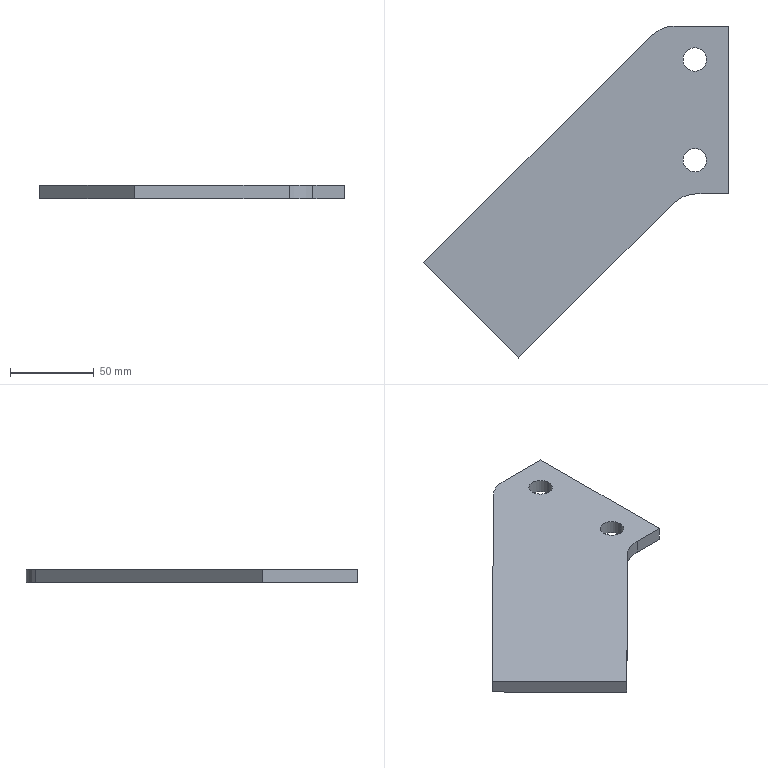Part | SolidWorks | features Extrusion 1 | 1 solid | 14 faces | box 181.644 x 197.856 x 8 mm | volume 132691 mm3 | plane 8 | cylinder 6 | commonest cylinder face diameters 14 x4 40 x2
STEP:
#1=CARTESIAN_POINT('',(-27.,-80.,8.));
#2=VERTEX_POINT('',#1);
#3=CARTESIAN_POINT('',(-13.,-80.,8.));
#4=VERTEX_POINT('',#3);
#5=CARTESIAN_POINT('',(-20.,-80.,8.));
#6=DIRECTION('',(0.,0.,1.));
#7=DIRECTION('',(1.,0.,0.));
#8=AXIS2_PLACEMENT_3D('',#5,#6,#7);
#9=CIRCLE('',#8,7.);
#10=EDGE_CURVE('',#2,#4,#9,.T.);
#11=ORIENTED_EDGE('',*,*,#10,.T.);
#12=CARTESIAN_POINT('',(-13.,-80.,0.));
#13=VERTEX_POINT('',#12);
#14=CARTESIAN_POINT('',(-13.,-80.,8.));
#15=DIRECTION('',(0.,0.,-1.));
#16=VECTOR('',#15,1000.);
#17=LINE('',#14,#16);
#18=EDGE_CURVE('',#4,#13,#17,.T.);
#19=ORIENTED_EDGE('',*,*,#18,.T.);
#20=CARTESIAN_POINT('',(-27.,-80.,0.));
#21=VERTEX_POINT('',#20);
#22=CARTESIAN_POINT('',(-20.,-80.,0.));
#23=DIRECTION('',(0.,0.,1.));
#24=DIRECTION('',(1.,0.,0.));
#25=AXIS2_PLACEMENT_3D('',#22,#23,#24);
#26=CIRCLE('',#25,7.);
#27=EDGE_CURVE('',#21,#13,#26,.T.);
#28=ORIENTED_EDGE('',*,*,#27,.F.);
#29=CARTESIAN_POINT('',(-27.,-80.,8.));
#30=DIRECTION('',(0.,0.,-1.));
#31=VECTOR('',#30,1000.);
#32=LINE('',#29,#31);
#33=EDGE_CURVE('',#2,#21,#32,.T.);
#34=ORIENTED_EDGE('',*,*,#33,.F.);
#35=EDGE_LOOP('',(#11,#19,#28,#34));
#36=FACE_OUTER_BOUND('',#35,.T.);
#37=CARTESIAN_POINT('',(-20.,-80.,8.));
#38=DIRECTION('',(0.,0.,-1.));
#39=DIRECTION('',(-1.,0.,0.));
#40=AXIS2_PLACEMENT_3D('',#37,#38,#39);
#41=CYLINDRICAL_SURFACE('',#40,7.);
#42=ADVANCED_FACE('',(#36),#41,.F.);
#43=CARTESIAN_POINT('',(-27.,-20.,8.));
#44=VERTEX_POINT('',#43);
#45=CARTESIAN_POINT('',(-13.,-20.,8.));
#46=VERTEX_POINT('',#45);
#47=CARTESIAN_POINT('',(-20.,-20.,8.));
#48=DIRECTION('',(0.,0.,1.));
#49=DIRECTION('',(1.,0.,0.));
#50=AXIS2_PLACEMENT_3D('',#47,#48,#49);
#51=CIRCLE('',#50,7.);
#52=EDGE_CURVE('',#44,#46,#51,.T.);
#53=ORIENTED_EDGE('',*,*,#52,.T.);
#54=CARTESIAN_POINT('',(-13.,-20.,0.));
#55=VERTEX_POINT('',#54);
#56=CARTESIAN_POINT('',(-13.,-20.,8.));
#57=DIRECTION('',(0.,0.,-1.));
#58=VECTOR('',#57,1000.);
#59=LINE('',#56,#58);
#60=EDGE_CURVE('',#46,#55,#59,.T.);
#61=ORIENTED_EDGE('',*,*,#60,.T.);
#62=CARTESIAN_POINT('',(-27.,-20.,0.));
#63=VERTEX_POINT('',#62);
#64=CARTESIAN_POINT('',(-20.,-20.,0.));
#65=DIRECTION('',(0.,0.,1.));
#66=DIRECTION('',(1.,0.,0.));
#67=AXIS2_PLACEMENT_3D('',#64,#65,#66);
#68=CIRCLE('',#67,7.);
#69=EDGE_CURVE('',#63,#55,#68,.T.);
#70=ORIENTED_EDGE('',*,*,#69,.F.);
#71=CARTESIAN_POINT('',(-27.,-20.,8.));
#72=DIRECTION('',(0.,0.,-1.));
#73=VECTOR('',#72,1000.);
#74=LINE('',#71,#73);
#75=EDGE_CURVE('',#44,#63,#74,.T.);
#76=ORIENTED_EDGE('',*,*,#75,.F.);
#77=EDGE_LOOP('',(#53,#61,#70,#76));
#78=FACE_OUTER_BOUND('',#77,.T.);
#79=CARTESIAN_POINT('',(-20.,-20.,8.));
#80=DIRECTION('',(0.,0.,-1.));
#81=DIRECTION('',(-1.,0.,0.));
#82=AXIS2_PLACEMENT_3D('',#79,#80,#81);
#83=CYLINDRICAL_SURFACE('',#82,7.);
#84=ADVANCED_FACE('',(#78),#83,.F.);
#85=CARTESIAN_POINT('',(0.,-100.,8.));
#86=VERTEX_POINT('',#85);
#87=CARTESIAN_POINT('',(0.,0.,8.));
#88=VERTEX_POINT('',#87);
#89=CARTESIAN_POINT('',(0.,0.,8.));
#90=DIRECTION('',(0.,1.,0.));
#91=VECTOR('',#90,1000.);
#92=LINE('',#89,#91);
#93=EDGE_CURVE('',#86,#88,#92,.T.);
#94=ORIENTED_EDGE('',*,*,#93,.T.);
#95=CARTESIAN_POINT('',(-31.734,0.,8.));
#96=VERTEX_POINT('',#95);
#97=CARTESIAN_POINT('',(0.,0.,8.));
#98=DIRECTION('',(-1.,0.,0.));
#99=VECTOR('',#98,1000.);
#100=LINE('',#97,#99);
#101=EDGE_CURVE('',#88,#96,#100,.T.);
#102=ORIENTED_EDGE('',*,*,#101,.T.);
#103=CARTESIAN_POINT('',(-45.854,-5.836,8.));
#104=VERTEX_POINT('',#103);
#105=CARTESIAN_POINT('',(-31.734,-20.,8.));
#106=DIRECTION('',(0.,0.,1.));
#107=DIRECTION('',(1.,0.,0.));
#108=AXIS2_PLACEMENT_3D('',#105,#106,#107);
#109=CIRCLE('',#108,20.);
#110=EDGE_CURVE('',#96,#104,#109,.T.);
#111=ORIENTED_EDGE('',*,*,#110,.T.);
#112=CARTESIAN_POINT('',(-181.644,-141.198,8.));
#113=VERTEX_POINT('',#112);
#114=CARTESIAN_POINT('',(-45.854,-5.836,8.));
#115=DIRECTION('',(-0.7082,-0.706,0.));
#116=VECTOR('',#115,1000.);
#117=LINE('',#114,#116);
#118=EDGE_CURVE('',#104,#113,#117,.T.);
#119=ORIENTED_EDGE('',*,*,#118,.T.);
#120=CARTESIAN_POINT('',(-125.165,-197.856,8.));
#121=VERTEX_POINT('',#120);
#122=CARTESIAN_POINT('',(-181.644,-141.198,8.));
#123=DIRECTION('',(0.706,-0.7082,0.));
#124=VECTOR('',#123,1000.);
#125=LINE('',#122,#124);
#126=EDGE_CURVE('',#113,#121,#125,.T.);
#127=ORIENTED_EDGE('',*,*,#126,.T.);
#128=CARTESIAN_POINT('',(-32.854,-105.836,8.));
#129=VERTEX_POINT('',#128);
#130=CARTESIAN_POINT('',(-125.165,-197.856,8.));
#131=DIRECTION('',(0.7082,0.706,0.));
#132=VECTOR('',#131,1000.);
#133=LINE('',#130,#132);
#134=EDGE_CURVE('',#121,#129,#133,.T.);
#135=ORIENTED_EDGE('',*,*,#134,.T.);
#136=CARTESIAN_POINT('',(-18.734,-100.,8.));
#137=VERTEX_POINT('',#136);
#138=CARTESIAN_POINT('',(-18.734,-120.,8.));
#139=DIRECTION('',(0.,0.,-1.));
#140=DIRECTION('',(-1.,0.,0.));
#141=AXIS2_PLACEMENT_3D('',#138,#139,#140);
#142=CIRCLE('',#141,20.);
#143=EDGE_CURVE('',#129,#137,#142,.T.);
#144=ORIENTED_EDGE('',*,*,#143,.T.);
#145=CARTESIAN_POINT('',(0.,-100.,8.));
#146=DIRECTION('',(1.,0.,0.));
#147=VECTOR('',#146,1000.);
#148=LINE('',#145,#147);
#149=EDGE_CURVE('',#137,#86,#148,.T.);
#150=ORIENTED_EDGE('',*,*,#149,.T.);
#151=EDGE_LOOP('',(#94,#102,#111,#119,#127,#135,#144,#150));
#152=FACE_OUTER_BOUND('',#151,.T.);
#153=ORIENTED_EDGE('',*,*,#52,.F.);
#154=CARTESIAN_POINT('',(-20.,-20.,8.));
#155=DIRECTION('',(0.,0.,1.));
#156=DIRECTION('',(1.,0.,0.));
#157=AXIS2_PLACEMENT_3D('',#154,#155,#156);
#158=CIRCLE('',#157,7.);
#159=EDGE_CURVE('',#46,#44,#158,.T.);
#160=ORIENTED_EDGE('',*,*,#159,.F.);
#161=EDGE_LOOP('',(#153,#160));
#162=FACE_BOUND('',#161,.T.);
#163=ORIENTED_EDGE('',*,*,#10,.F.);
#164=CARTESIAN_POINT('',(-20.,-80.,8.));
#165=DIRECTION('',(0.,0.,1.));
#166=DIRECTION('',(1.,0.,0.));
#167=AXIS2_PLACEMENT_3D('',#164,#165,#166);
#168=CIRCLE('',#167,7.);
#169=EDGE_CURVE('',#4,#2,#168,.T.);
#170=ORIENTED_EDGE('',*,*,#169,.F.);
#171=EDGE_LOOP('',(#163,#170));
#172=FACE_BOUND('',#171,.T.);
#173=CARTESIAN_POINT('',(-18.734,-120.,8.));
#174=DIRECTION('',(0.,0.,-1.));
#175=DIRECTION('',(-1.,0.,0.));
#176=AXIS2_PLACEMENT_3D('',#173,#174,#175);
#177=PLANE('',#176);
#178=ADVANCED_FACE('',(#152,#162,#172),#177,.F.);
#179=ORIENTED_EDGE('',*,*,#69,.T.);
#180=CARTESIAN_POINT('',(-20.,-20.,0.));
#181=DIRECTION('',(0.,0.,1.));
#182=DIRECTION('',(1.,0.,0.));
#183=AXIS2_PLACEMENT_3D('',#180,#181,#182);
#184=CIRCLE('',#183,7.);
#185=EDGE_CURVE('',#55,#63,#184,.T.);
#186=ORIENTED_EDGE('',*,*,#185,.T.);
#187=EDGE_LOOP('',(#179,#186));
#188=FACE_BOUND('',#187,.T.);
#189=CARTESIAN_POINT('',(0.,-100.,0.));
#190=VERTEX_POINT('',#189);
#191=CARTESIAN_POINT('',(0.,0.,0.));
#192=VERTEX_POINT('',#191);
#193=CARTESIAN_POINT('',(0.,0.,0.));
#194=DIRECTION('',(0.,1.,0.));
#195=VECTOR('',#194,1000.);
#196=LINE('',#193,#195);
#197=EDGE_CURVE('',#190,#192,#196,.T.);
#198=ORIENTED_EDGE('',*,*,#197,.F.);
#199=CARTESIAN_POINT('',(-18.734,-100.,0.));
#200=VERTEX_POINT('',#199);
#201=CARTESIAN_POINT('',(0.,-100.,0.));
#202=DIRECTION('',(1.,0.,0.));
#203=VECTOR('',#202,1000.);
#204=LINE('',#201,#203);
#205=EDGE_CURVE('',#200,#190,#204,.T.);
#206=ORIENTED_EDGE('',*,*,#205,.F.);
#207=CARTESIAN_POINT('',(-32.854,-105.836,0.));
#208=VERTEX_POINT('',#207);
#209=CARTESIAN_POINT('',(-18.734,-120.,0.));
#210=DIRECTION('',(0.,0.,-1.));
#211=DIRECTION('',(-1.,0.,0.));
#212=AXIS2_PLACEMENT_3D('',#209,#210,#211);
#213=CIRCLE('',#212,20.);
#214=EDGE_CURVE('',#208,#200,#213,.T.);
#215=ORIENTED_EDGE('',*,*,#214,.F.);
#216=CARTESIAN_POINT('',(-125.165,-197.856,0.));
#217=VERTEX_POINT('',#216);
#218=CARTESIAN_POINT('',(-125.165,-197.856,0.));
#219=DIRECTION('',(0.7082,0.706,0.));
#220=VECTOR('',#219,1000.);
#221=LINE('',#218,#220);
#222=EDGE_CURVE('',#217,#208,#221,.T.);
#223=ORIENTED_EDGE('',*,*,#222,.F.);
#224=CARTESIAN_POINT('',(-181.644,-141.198,0.));
#225=VERTEX_POINT('',#224);
#226=CARTESIAN_POINT('',(-181.644,-141.198,0.));
#227=DIRECTION('',(0.706,-0.7082,0.));
#228=VECTOR('',#227,1000.);
#229=LINE('',#226,#228);
#230=EDGE_CURVE('',#225,#217,#229,.T.);
#231=ORIENTED_EDGE('',*,*,#230,.F.);
#232=CARTESIAN_POINT('',(-45.854,-5.836,0.));
#233=VERTEX_POINT('',#232);
#234=CARTESIAN_POINT('',(-45.854,-5.836,0.));
#235=DIRECTION('',(-0.7082,-0.706,0.));
#236=VECTOR('',#235,1000.);
#237=LINE('',#234,#236);
#238=EDGE_CURVE('',#233,#225,#237,.T.);
#239=ORIENTED_EDGE('',*,*,#238,.F.);
#240=CARTESIAN_POINT('',(-31.734,0.,0.));
#241=VERTEX_POINT('',#240);
#242=CARTESIAN_POINT('',(-31.734,-20.,0.));
#243=DIRECTION('',(0.,0.,1.));
#244=DIRECTION('',(1.,0.,0.));
#245=AXIS2_PLACEMENT_3D('',#242,#243,#244);
#246=CIRCLE('',#245,20.);
#247=EDGE_CURVE('',#241,#233,#246,.T.);
#248=ORIENTED_EDGE('',*,*,#247,.F.);
#249=CARTESIAN_POINT('',(0.,0.,0.));
#250=DIRECTION('',(-1.,0.,0.));
#251=VECTOR('',#250,1000.);
#252=LINE('',#249,#251);
#253=EDGE_CURVE('',#192,#241,#252,.T.);
#254=ORIENTED_EDGE('',*,*,#253,.F.);
#255=EDGE_LOOP('',(#198,#206,#215,#223,#231,#239,#248,#254));
#256=FACE_OUTER_BOUND('',#255,.T.);
#257=ORIENTED_EDGE('',*,*,#27,.T.);
#258=CARTESIAN_POINT('',(-20.,-80.,0.));
#259=DIRECTION('',(0.,0.,1.));
#260=DIRECTION('',(1.,0.,0.));
#261=AXIS2_PLACEMENT_3D('',#258,#259,#260);
#262=CIRCLE('',#261,7.);
#263=EDGE_CURVE('',#13,#21,#262,.T.);
#264=ORIENTED_EDGE('',*,*,#263,.T.);
#265=EDGE_LOOP('',(#257,#264));
#266=FACE_BOUND('',#265,.T.);
#267=CARTESIAN_POINT('',(-18.734,-120.,0.));
#268=DIRECTION('',(0.,0.,-1.));
#269=DIRECTION('',(-1.,0.,0.));
#270=AXIS2_PLACEMENT_3D('',#267,#268,#269);
#271=PLANE('',#270);
#272=ADVANCED_FACE('',(#188,#256,#266),#271,.T.);
#273=ORIENTED_EDGE('',*,*,#197,.T.);
#274=CARTESIAN_POINT('',(0.,0.,8.));
#275=DIRECTION('',(0.,0.,-1.));
#276=VECTOR('',#275,1000.);
#277=LINE('',#274,#276);
#278=EDGE_CURVE('',#88,#192,#277,.T.);
#279=ORIENTED_EDGE('',*,*,#278,.F.);
#280=ORIENTED_EDGE('',*,*,#93,.F.);
#281=CARTESIAN_POINT('',(0.,-100.,8.));
#282=DIRECTION('',(0.,0.,-1.));
#283=VECTOR('',#282,1000.);
#284=LINE('',#281,#283);
#285=EDGE_CURVE('',#86,#190,#284,.T.);
#286=ORIENTED_EDGE('',*,*,#285,.T.);
#287=EDGE_LOOP('',(#273,#279,#280,#286));
#288=FACE_OUTER_BOUND('',#287,.T.);
#289=CARTESIAN_POINT('',(0.,0.,8.));
#290=DIRECTION('',(-1.,0.,0.));
#291=DIRECTION('',(0.,-1.,0.));
#292=AXIS2_PLACEMENT_3D('',#289,#290,#291);
#293=PLANE('',#292);
#294=ADVANCED_FACE('',(#288),#293,.F.);
#295=ORIENTED_EDGE('',*,*,#253,.T.);
#296=CARTESIAN_POINT('',(-31.734,0.,8.));
#297=DIRECTION('',(0.,0.,-1.));
#298=VECTOR('',#297,1000.);
#299=LINE('',#296,#298);
#300=EDGE_CURVE('',#96,#241,#299,.T.);
#301=ORIENTED_EDGE('',*,*,#300,.F.);
#302=ORIENTED_EDGE('',*,*,#101,.F.);
#303=ORIENTED_EDGE('',*,*,#278,.T.);
#304=EDGE_LOOP('',(#295,#301,#302,#303));
#305=FACE_OUTER_BOUND('',#304,.T.);
#306=CARTESIAN_POINT('',(0.,0.,8.));
#307=DIRECTION('',(0.,-1.,0.));
#308=DIRECTION('',(0.,0.,-1.));
#309=AXIS2_PLACEMENT_3D('',#306,#307,#308);
#310=PLANE('',#309);
#311=ADVANCED_FACE('',(#305),#310,.F.);
#312=ORIENTED_EDGE('',*,*,#247,.T.);
#313=CARTESIAN_POINT('',(-45.854,-5.836,8.));
#314=DIRECTION('',(0.,0.,-1.));
#315=VECTOR('',#314,1000.);
#316=LINE('',#313,#315);
#317=EDGE_CURVE('',#104,#233,#316,.T.);
#318=ORIENTED_EDGE('',*,*,#317,.F.);
#319=ORIENTED_EDGE('',*,*,#110,.F.);
#320=ORIENTED_EDGE('',*,*,#300,.T.);
#321=EDGE_LOOP('',(#312,#318,#319,#320));
#322=FACE_OUTER_BOUND('',#321,.T.);
#323=CARTESIAN_POINT('',(-31.734,-20.,8.));
#324=DIRECTION('',(0.,0.,-1.));
#325=DIRECTION('',(-1.,0.,0.));
#326=AXIS2_PLACEMENT_3D('',#323,#324,#325);
#327=CYLINDRICAL_SURFACE('',#326,20.);
#328=ADVANCED_FACE('',(#322),#327,.T.);
#329=ORIENTED_EDGE('',*,*,#238,.T.);
#330=CARTESIAN_POINT('',(-181.644,-141.198,8.));
#331=DIRECTION('',(0.,0.,-1.));
#332=VECTOR('',#331,1000.);
#333=LINE('',#330,#332);
#334=EDGE_CURVE('',#113,#225,#333,.T.);
#335=ORIENTED_EDGE('',*,*,#334,.F.);
#336=ORIENTED_EDGE('',*,*,#118,.F.);
#337=ORIENTED_EDGE('',*,*,#317,.T.);
#338=EDGE_LOOP('',(#329,#335,#336,#337));
#339=FACE_OUTER_BOUND('',#338,.T.);
#340=CARTESIAN_POINT('',(-45.854,-5.836,8.));
#341=DIRECTION('',(0.706,-0.7082,0.));
#342=DIRECTION('',(0.7082,0.706,0.));
#343=AXIS2_PLACEMENT_3D('',#340,#341,#342);
#344=PLANE('',#343);
#345=ADVANCED_FACE('',(#339),#344,.F.);
#346=ORIENTED_EDGE('',*,*,#230,.T.);
#347=CARTESIAN_POINT('',(-125.165,-197.856,8.));
#348=DIRECTION('',(0.,0.,-1.));
#349=VECTOR('',#348,1000.);
#350=LINE('',#347,#349);
#351=EDGE_CURVE('',#121,#217,#350,.T.);
#352=ORIENTED_EDGE('',*,*,#351,.F.);
#353=ORIENTED_EDGE('',*,*,#126,.F.);
#354=ORIENTED_EDGE('',*,*,#334,.T.);
#355=EDGE_LOOP('',(#346,#352,#353,#354));
#356=FACE_OUTER_BOUND('',#355,.T.);
#357=CARTESIAN_POINT('',(-181.644,-141.198,8.));
#358=DIRECTION('',(0.7082,0.706,0.));
#359=DIRECTION('',(-0.706,0.7082,0.));
#360=AXIS2_PLACEMENT_3D('',#357,#358,#359);
#361=PLANE('',#360);
#362=ADVANCED_FACE('',(#356),#361,.F.);
#363=ORIENTED_EDGE('',*,*,#222,.T.);
#364=CARTESIAN_POINT('',(-32.854,-105.836,8.));
#365=DIRECTION('',(0.,0.,-1.));
#366=VECTOR('',#365,1000.);
#367=LINE('',#364,#366);
#368=EDGE_CURVE('',#129,#208,#367,.T.);
#369=ORIENTED_EDGE('',*,*,#368,.F.);
#370=ORIENTED_EDGE('',*,*,#134,.F.);
#371=ORIENTED_EDGE('',*,*,#351,.T.);
#372=EDGE_LOOP('',(#363,#369,#370,#371));
#373=FACE_OUTER_BOUND('',#372,.T.);
#374=CARTESIAN_POINT('',(-125.165,-197.856,8.));
#375=DIRECTION('',(-0.706,0.7082,0.));
#376=DIRECTION('',(-0.7082,-0.706,0.));
#377=AXIS2_PLACEMENT_3D('',#374,#375,#376);
#378=PLANE('',#377);
#379=ADVANCED_FACE('',(#373),#378,.F.);
#380=ORIENTED_EDGE('',*,*,#214,.T.);
#381=CARTESIAN_POINT('',(-18.734,-100.,8.));
#382=DIRECTION('',(0.,0.,-1.));
#383=VECTOR('',#382,1000.);
#384=LINE('',#381,#383);
#385=EDGE_CURVE('',#137,#200,#384,.T.);
#386=ORIENTED_EDGE('',*,*,#385,.F.);
#387=ORIENTED_EDGE('',*,*,#143,.F.);
#388=ORIENTED_EDGE('',*,*,#368,.T.);
#389=EDGE_LOOP('',(#380,#386,#387,#388));
#390=FACE_OUTER_BOUND('',#389,.T.);
#391=CARTESIAN_POINT('',(-18.734,-120.,8.));
#392=DIRECTION('',(0.,0.,-1.));
#393=DIRECTION('',(-1.,0.,0.));
#394=AXIS2_PLACEMENT_3D('',#391,#392,#393);
#395=CYLINDRICAL_SURFACE('',#394,20.);
#396=ADVANCED_FACE('',(#390),#395,.F.);
#397=ORIENTED_EDGE('',*,*,#205,.T.);
#398=ORIENTED_EDGE('',*,*,#285,.F.);
#399=ORIENTED_EDGE('',*,*,#149,.F.);
#400=ORIENTED_EDGE('',*,*,#385,.T.);
#401=EDGE_LOOP('',(#397,#398,#399,#400));
#402=FACE_OUTER_BOUND('',#401,.T.);
#403=CARTESIAN_POINT('',(0.,-100.,8.));
#404=DIRECTION('',(0.,1.,0.));
#405=DIRECTION('',(0.,0.,1.));
#406=AXIS2_PLACEMENT_3D('',#403,#404,#405);
#407=PLANE('',#406);
#408=ADVANCED_FACE('',(#402),#407,.F.);
#409=ORIENTED_EDGE('',*,*,#60,.F.);
#410=ORIENTED_EDGE('',*,*,#159,.T.);
#411=ORIENTED_EDGE('',*,*,#75,.T.);
#412=ORIENTED_EDGE('',*,*,#185,.F.);
#413=EDGE_LOOP('',(#409,#410,#411,#412));
#414=FACE_OUTER_BOUND('',#413,.T.);
#415=CARTESIAN_POINT('',(-20.,-20.,8.));
#416=DIRECTION('',(0.,0.,-1.));
#417=DIRECTION('',(-1.,0.,0.));
#418=AXIS2_PLACEMENT_3D('',#415,#416,#417);
#419=CYLINDRICAL_SURFACE('',#418,7.);
#420=ADVANCED_FACE('',(#414),#419,.F.);
#421=ORIENTED_EDGE('',*,*,#18,.F.);
#422=ORIENTED_EDGE('',*,*,#169,.T.);
#423=ORIENTED_EDGE('',*,*,#33,.T.);
#424=ORIENTED_EDGE('',*,*,#263,.F.);
#425=EDGE_LOOP('',(#421,#422,#423,#424));
#426=FACE_OUTER_BOUND('',#425,.T.);
#427=CARTESIAN_POINT('',(-20.,-80.,8.));
#428=DIRECTION('',(0.,0.,-1.));
#429=DIRECTION('',(-1.,0.,0.));
#430=AXIS2_PLACEMENT_3D('',#427,#428,#429);
#431=CYLINDRICAL_SURFACE('',#430,7.);
#432=ADVANCED_FACE('',(#426),#431,.F.);
#433=CLOSED_SHELL('',(#42,#84,#178,#272,#294,#311,#328,#345,#362,#379,#396,#408,#420,#432));
#434=MANIFOLD_SOLID_BREP('',#433);
#435=CARTESIAN_POINT('',(0.,0.,0.));
#436=DIRECTION('',(0.,0.,1.));
#437=DIRECTION('',(1.,0.,0.));
#438=AXIS2_PLACEMENT_3D('',#435,#436,#437);
#439=(LENGTH_UNIT()NAMED_UNIT(*)SI_UNIT(.MILLI.,.METRE.));
#440=UNCERTAINTY_MEASURE_WITH_UNIT(LENGTH_MEASURE(0.00001),#439,'','');
#441=(NAMED_UNIT(*)PLANE_ANGLE_UNIT()SI_UNIT($,.RADIAN.));
#442=(NAMED_UNIT(*)SI_UNIT($,.STERADIAN.)SOLID_ANGLE_UNIT());
#443=(GEOMETRIC_REPRESENTATION_CONTEXT(3)GLOBAL_UNCERTAINTY_ASSIGNED_CONTEXT((#440))GLOBAL_UNIT_ASSIGNED_CONTEXT((#439,#441,#442))REPRESENTATION_CONTEXT('',''));
#444=ADVANCED_BREP_SHAPE_REPRESENTATION('',(#434,#438),#443);